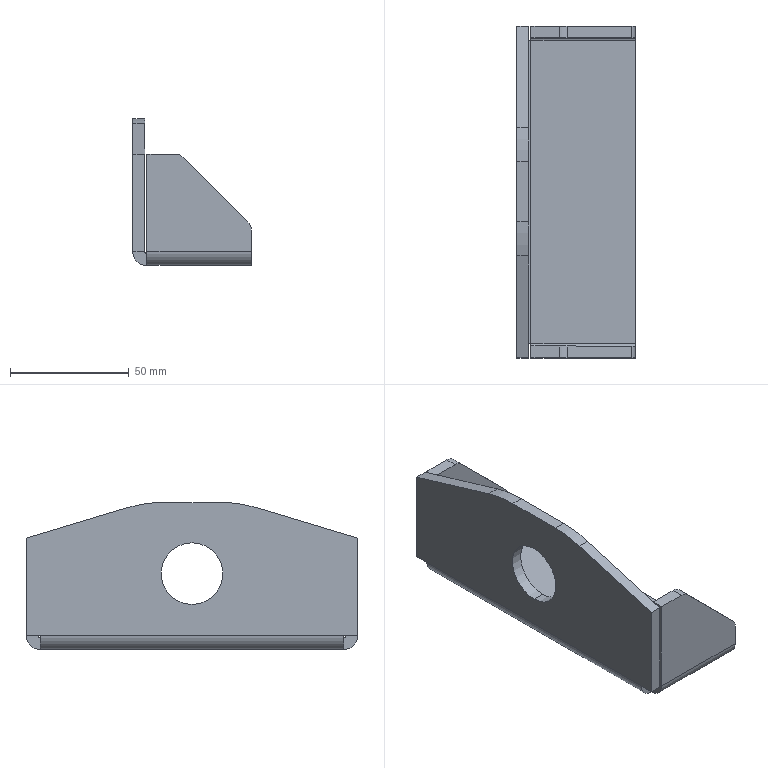Part | SolidWorks | features BaseBody 1 | 1 solid | 44 faces | box 50 x 140 x 62 mm | volume 80396 mm3 | plane 30 | cylinder 14 | commonest cylinder face diameters 10 x4 2 x3 12 x3 26 x2 100 x2
STEP:
#1=CARTESIAN_POINT('',(-20.,0.,14.));
#2=VERTEX_POINT('',#1);
#3=CARTESIAN_POINT('',(-25.,0.,14.));
#4=VERTEX_POINT('',#3);
#5=CARTESIAN_POINT('',(-20.,0.,14.));
#6=DIRECTION('',(-1.,0.,0.));
#7=VECTOR('',#6,1000.);
#8=LINE('',#5,#7);
#9=EDGE_CURVE('',#2,#4,#8,.T.);
#10=ORIENTED_EDGE('',*,*,#9,.F.);
#11=CARTESIAN_POINT('',(-20.,0.,40.));
#12=VERTEX_POINT('',#11);
#13=CARTESIAN_POINT('',(-20.,0.,27.));
#14=DIRECTION('',(-1.,0.,0.));
#15=DIRECTION('',(0.,0.,1.));
#16=AXIS2_PLACEMENT_3D('',#13,#14,#15);
#17=CIRCLE('',#16,13.);
#18=EDGE_CURVE('',#12,#2,#17,.T.);
#19=ORIENTED_EDGE('',*,*,#18,.F.);
#20=CARTESIAN_POINT('',(-25.,0.,40.));
#21=VERTEX_POINT('',#20);
#22=CARTESIAN_POINT('',(-20.,0.,40.));
#23=DIRECTION('',(-1.,0.,0.));
#24=VECTOR('',#23,1000.);
#25=LINE('',#22,#24);
#26=EDGE_CURVE('',#12,#21,#25,.T.);
#27=ORIENTED_EDGE('',*,*,#26,.T.);
#28=CARTESIAN_POINT('',(-25.,0.,27.));
#29=DIRECTION('',(-1.,0.,0.));
#30=DIRECTION('',(0.,0.,1.));
#31=AXIS2_PLACEMENT_3D('',#28,#29,#30);
#32=CIRCLE('',#31,13.);
#33=EDGE_CURVE('',#21,#4,#32,.T.);
#34=ORIENTED_EDGE('',*,*,#33,.T.);
#35=EDGE_LOOP('',(#10,#19,#27,#34));
#36=FACE_OUTER_BOUND('',#35,.T.);
#37=CARTESIAN_POINT('',(-20.,0.,27.));
#38=DIRECTION('',(-1.,0.,0.));
#39=DIRECTION('',(0.,0.,1.));
#40=AXIS2_PLACEMENT_3D('',#37,#38,#39);
#41=CYLINDRICAL_SURFACE('',#40,13.);
#42=ADVANCED_FACE('',(#36),#41,.F.);
#43=CARTESIAN_POINT('',(-3.536,-70.,40.536));
#44=VERTEX_POINT('',#43);
#45=CARTESIAN_POINT('',(-7.071,-70.,42.));
#46=VERTEX_POINT('',#45);
#47=CARTESIAN_POINT('',(-7.071,-70.,37.));
#48=DIRECTION('',(0.,-1.,0.));
#49=DIRECTION('',(0.,0.,1.));
#50=AXIS2_PLACEMENT_3D('',#47,#48,#49);
#51=CIRCLE('',#50,5.);
#52=EDGE_CURVE('',#44,#46,#51,.T.);
#53=ORIENTED_EDGE('',*,*,#52,.F.);
#54=CARTESIAN_POINT('',(-3.536,-65.,40.536));
#55=VERTEX_POINT('',#54);
#56=CARTESIAN_POINT('',(-3.536,-70.,40.536));
#57=DIRECTION('',(0.,-1.,0.));
#58=VECTOR('',#57,1000.);
#59=LINE('',#56,#58);
#60=EDGE_CURVE('',#55,#44,#59,.T.);
#61=ORIENTED_EDGE('',*,*,#60,.F.);
#62=CARTESIAN_POINT('',(-7.071,-65.,42.));
#63=VERTEX_POINT('',#62);
#64=CARTESIAN_POINT('',(-7.071,-65.,37.));
#65=DIRECTION('',(0.,1.,0.));
#66=DIRECTION('',(0.,0.,1.));
#67=AXIS2_PLACEMENT_3D('',#64,#65,#66);
#68=CIRCLE('',#67,5.);
#69=EDGE_CURVE('',#63,#55,#68,.T.);
#70=ORIENTED_EDGE('',*,*,#69,.F.);
#71=CARTESIAN_POINT('',(-7.071,-65.,42.));
#72=DIRECTION('',(0.,1.,0.));
#73=VECTOR('',#72,1000.);
#74=LINE('',#71,#73);
#75=EDGE_CURVE('',#46,#63,#74,.T.);
#76=ORIENTED_EDGE('',*,*,#75,.F.);
#77=EDGE_LOOP('',(#53,#61,#70,#76));
#78=FACE_OUTER_BOUND('',#77,.T.);
#79=CARTESIAN_POINT('',(-7.071,-70.,37.));
#80=DIRECTION('',(0.,1.,0.));
#81=DIRECTION('',(0.,0.,1.));
#82=AXIS2_PLACEMENT_3D('',#79,#80,#81);
#83=CYLINDRICAL_SURFACE('',#82,5.);
#84=ADVANCED_FACE('',(#78),#83,.T.);
#85=CARTESIAN_POINT('',(23.536,-65.,13.464));
#86=VERTEX_POINT('',#85);
#87=CARTESIAN_POINT('',(25.,-65.,9.929));
#88=VERTEX_POINT('',#87);
#89=CARTESIAN_POINT('',(20.,-65.,9.929));
#90=DIRECTION('',(0.,1.,0.));
#91=DIRECTION('',(0.,0.,1.));
#92=AXIS2_PLACEMENT_3D('',#89,#90,#91);
#93=CIRCLE('',#92,5.);
#94=EDGE_CURVE('',#86,#88,#93,.T.);
#95=ORIENTED_EDGE('',*,*,#94,.F.);
#96=CARTESIAN_POINT('',(23.536,-70.,13.464));
#97=VERTEX_POINT('',#96);
#98=CARTESIAN_POINT('',(23.536,-65.,13.464));
#99=DIRECTION('',(0.,1.,0.));
#100=VECTOR('',#99,1000.);
#101=LINE('',#98,#100);
#102=EDGE_CURVE('',#97,#86,#101,.T.);
#103=ORIENTED_EDGE('',*,*,#102,.F.);
#104=CARTESIAN_POINT('',(25.,-70.,9.929));
#105=VERTEX_POINT('',#104);
#106=CARTESIAN_POINT('',(20.,-70.,9.929));
#107=DIRECTION('',(0.,-1.,0.));
#108=DIRECTION('',(0.,0.,1.));
#109=AXIS2_PLACEMENT_3D('',#106,#107,#108);
#110=CIRCLE('',#109,5.);
#111=EDGE_CURVE('',#105,#97,#110,.T.);
#112=ORIENTED_EDGE('',*,*,#111,.F.);
#113=CARTESIAN_POINT('',(25.,-70.,9.929));
#114=DIRECTION('',(0.,-1.,0.));
#115=VECTOR('',#114,1000.);
#116=LINE('',#113,#115);
#117=EDGE_CURVE('',#88,#105,#116,.T.);
#118=ORIENTED_EDGE('',*,*,#117,.F.);
#119=EDGE_LOOP('',(#95,#103,#112,#118));
#120=FACE_OUTER_BOUND('',#119,.T.);
#121=CARTESIAN_POINT('',(20.,-70.,9.929));
#122=DIRECTION('',(0.,-1.,0.));
#123=DIRECTION('',(0.,0.,-1.));
#124=AXIS2_PLACEMENT_3D('',#121,#122,#123);
#125=CYLINDRICAL_SURFACE('',#124,5.);
#126=ADVANCED_FACE('',(#120),#125,.T.);
#127=CARTESIAN_POINT('',(23.536,70.,13.464));
#128=VERTEX_POINT('',#127);
#129=CARTESIAN_POINT('',(25.,70.,9.929));
#130=VERTEX_POINT('',#129);
#131=CARTESIAN_POINT('',(20.,70.,9.929));
#132=DIRECTION('',(0.,1.,0.));
#133=DIRECTION('',(0.,0.,-1.));
#134=AXIS2_PLACEMENT_3D('',#131,#132,#133);
#135=CIRCLE('',#134,5.);
#136=EDGE_CURVE('',#128,#130,#135,.T.);
#137=ORIENTED_EDGE('',*,*,#136,.F.);
#138=CARTESIAN_POINT('',(23.536,65.,13.464));
#139=VERTEX_POINT('',#138);
#140=CARTESIAN_POINT('',(23.536,70.,13.464));
#141=DIRECTION('',(0.,1.,0.));
#142=VECTOR('',#141,1000.);
#143=LINE('',#140,#142);
#144=EDGE_CURVE('',#139,#128,#143,.T.);
#145=ORIENTED_EDGE('',*,*,#144,.F.);
#146=CARTESIAN_POINT('',(25.,65.,9.929));
#147=VERTEX_POINT('',#146);
#148=CARTESIAN_POINT('',(20.,65.,9.929));
#149=DIRECTION('',(0.,-1.,0.));
#150=DIRECTION('',(0.,0.,-1.));
#151=AXIS2_PLACEMENT_3D('',#148,#149,#150);
#152=CIRCLE('',#151,5.);
#153=EDGE_CURVE('',#147,#139,#152,.T.);
#154=ORIENTED_EDGE('',*,*,#153,.F.);
#155=CARTESIAN_POINT('',(25.,65.,9.929));
#156=DIRECTION('',(0.,-1.,0.));
#157=VECTOR('',#156,1000.);
#158=LINE('',#155,#157);
#159=EDGE_CURVE('',#130,#147,#158,.T.);
#160=ORIENTED_EDGE('',*,*,#159,.F.);
#161=EDGE_LOOP('',(#137,#145,#154,#160));
#162=FACE_OUTER_BOUND('',#161,.T.);
#163=CARTESIAN_POINT('',(20.,70.,9.929));
#164=DIRECTION('',(0.,-1.,0.));
#165=DIRECTION('',(0.,0.,-1.));
#166=AXIS2_PLACEMENT_3D('',#163,#164,#165);
#167=CYLINDRICAL_SURFACE('',#166,5.);
#168=ADVANCED_FACE('',(#162),#167,.T.);
#169=CARTESIAN_POINT('',(-3.536,65.,40.536));
#170=VERTEX_POINT('',#169);
#171=CARTESIAN_POINT('',(-7.071,65.,42.));
#172=VERTEX_POINT('',#171);
#173=CARTESIAN_POINT('',(-7.071,65.,37.));
#174=DIRECTION('',(0.,-1.,0.));
#175=DIRECTION('',(0.,0.,-1.));
#176=AXIS2_PLACEMENT_3D('',#173,#174,#175);
#177=CIRCLE('',#176,5.);
#178=EDGE_CURVE('',#170,#172,#177,.T.);
#179=ORIENTED_EDGE('',*,*,#178,.F.);
#180=CARTESIAN_POINT('',(-3.536,70.,40.536));
#181=VERTEX_POINT('',#180);
#182=CARTESIAN_POINT('',(-3.536,65.,40.536));
#183=DIRECTION('',(0.,-1.,0.));
#184=VECTOR('',#183,1000.);
#185=LINE('',#182,#184);
#186=EDGE_CURVE('',#181,#170,#185,.T.);
#187=ORIENTED_EDGE('',*,*,#186,.F.);
#188=CARTESIAN_POINT('',(-7.071,70.,42.));
#189=VERTEX_POINT('',#188);
#190=CARTESIAN_POINT('',(-7.071,70.,37.));
#191=DIRECTION('',(0.,1.,0.));
#192=DIRECTION('',(0.,0.,-1.));
#193=AXIS2_PLACEMENT_3D('',#190,#191,#192);
#194=CIRCLE('',#193,5.);
#195=EDGE_CURVE('',#189,#181,#194,.T.);
#196=ORIENTED_EDGE('',*,*,#195,.F.);
#197=CARTESIAN_POINT('',(-7.071,70.,42.));
#198=DIRECTION('',(0.,1.,0.));
#199=VECTOR('',#198,1000.);
#200=LINE('',#197,#199);
#201=EDGE_CURVE('',#172,#189,#200,.T.);
#202=ORIENTED_EDGE('',*,*,#201,.F.);
#203=EDGE_LOOP('',(#179,#187,#196,#202));
#204=FACE_OUTER_BOUND('',#203,.T.);
#205=CARTESIAN_POINT('',(-7.071,70.,37.));
#206=DIRECTION('',(0.,1.,0.));
#207=DIRECTION('',(0.,0.,1.));
#208=AXIS2_PLACEMENT_3D('',#205,#206,#207);
#209=CYLINDRICAL_SURFACE('',#208,5.);
#210=ADVANCED_FACE('',(#204),#209,.T.);
#211=CARTESIAN_POINT('',(-25.,-27.029,54.891));
#212=VERTEX_POINT('',#211);
#213=CARTESIAN_POINT('',(-25.,-12.662,57.));
#214=VERTEX_POINT('',#213);
#215=CARTESIAN_POINT('',(-25.,-12.662,7.));
#216=DIRECTION('',(-1.,0.,0.));
#217=DIRECTION('',(0.,0.,-1.));
#218=AXIS2_PLACEMENT_3D('',#215,#216,#217);
#219=CIRCLE('',#218,50.);
#220=EDGE_CURVE('',#212,#214,#219,.T.);
#221=ORIENTED_EDGE('',*,*,#220,.F.);
#222=CARTESIAN_POINT('',(-20.,-27.029,54.891));
#223=VERTEX_POINT('',#222);
#224=CARTESIAN_POINT('',(-25.,-27.029,54.891));
#225=DIRECTION('',(-1.,0.,0.));
#226=VECTOR('',#225,1000.);
#227=LINE('',#224,#226);
#228=EDGE_CURVE('',#223,#212,#227,.T.);
#229=ORIENTED_EDGE('',*,*,#228,.F.);
#230=CARTESIAN_POINT('',(-20.,-12.662,57.));
#231=VERTEX_POINT('',#230);
#232=CARTESIAN_POINT('',(-20.,-12.662,7.));
#233=DIRECTION('',(1.,0.,0.));
#234=DIRECTION('',(0.,0.,-1.));
#235=AXIS2_PLACEMENT_3D('',#232,#233,#234);
#236=CIRCLE('',#235,50.);
#237=EDGE_CURVE('',#231,#223,#236,.T.);
#238=ORIENTED_EDGE('',*,*,#237,.F.);
#239=CARTESIAN_POINT('',(-20.,-12.662,57.));
#240=DIRECTION('',(1.,0.,0.));
#241=VECTOR('',#240,1000.);
#242=LINE('',#239,#241);
#243=EDGE_CURVE('',#214,#231,#242,.T.);
#244=ORIENTED_EDGE('',*,*,#243,.F.);
#245=EDGE_LOOP('',(#221,#229,#238,#244));
#246=FACE_OUTER_BOUND('',#245,.T.);
#247=CARTESIAN_POINT('',(-25.,-12.662,7.));
#248=DIRECTION('',(1.,0.,0.));
#249=DIRECTION('',(0.,0.,-1.));
#250=AXIS2_PLACEMENT_3D('',#247,#248,#249);
#251=CYLINDRICAL_SURFACE('',#250,50.);
#252=ADVANCED_FACE('',(#246),#251,.T.);
#253=CARTESIAN_POINT('',(-20.,27.029,54.891));
#254=VERTEX_POINT('',#253);
#255=CARTESIAN_POINT('',(-20.,12.662,57.));
#256=VERTEX_POINT('',#255);
#257=CARTESIAN_POINT('',(-20.,12.662,7.));
#258=DIRECTION('',(1.,0.,0.));
#259=DIRECTION('',(0.,0.,-1.));
#260=AXIS2_PLACEMENT_3D('',#257,#258,#259);
#261=CIRCLE('',#260,50.);
#262=EDGE_CURVE('',#254,#256,#261,.T.);
#263=ORIENTED_EDGE('',*,*,#262,.F.);
#264=CARTESIAN_POINT('',(-25.,27.029,54.891));
#265=VERTEX_POINT('',#264);
#266=CARTESIAN_POINT('',(-20.,27.029,54.891));
#267=DIRECTION('',(1.,0.,0.));
#268=VECTOR('',#267,1000.);
#269=LINE('',#266,#268);
#270=EDGE_CURVE('',#265,#254,#269,.T.);
#271=ORIENTED_EDGE('',*,*,#270,.F.);
#272=CARTESIAN_POINT('',(-25.,12.662,57.));
#273=VERTEX_POINT('',#272);
#274=CARTESIAN_POINT('',(-25.,12.662,7.));
#275=DIRECTION('',(-1.,0.,0.));
#276=DIRECTION('',(0.,0.,-1.));
#277=AXIS2_PLACEMENT_3D('',#274,#275,#276);
#278=CIRCLE('',#277,50.);
#279=EDGE_CURVE('',#273,#265,#278,.T.);
#280=ORIENTED_EDGE('',*,*,#279,.F.);
#281=CARTESIAN_POINT('',(-25.,12.662,57.));
#282=DIRECTION('',(-1.,0.,0.));
#283=VECTOR('',#282,1000.);
#284=LINE('',#281,#283);
#285=EDGE_CURVE('',#256,#273,#284,.T.);
#286=ORIENTED_EDGE('',*,*,#285,.F.);
#287=EDGE_LOOP('',(#263,#271,#280,#286));
#288=FACE_OUTER_BOUND('',#287,.T.);
#289=CARTESIAN_POINT('',(-25.,12.662,7.));
#290=DIRECTION('',(-1.,0.,0.));
#291=DIRECTION('',(0.,0.,1.));
#292=AXIS2_PLACEMENT_3D('',#289,#290,#291);
#293=CYLINDRICAL_SURFACE('',#292,50.);
#294=ADVANCED_FACE('',(#288),#293,.T.);
#295=CARTESIAN_POINT('',(-20.,-70.,42.));
#296=VERTEX_POINT('',#295);
#297=CARTESIAN_POINT('',(-20.,-17.339,57.798));
#298=DIRECTION('',(0.,-0.9578,-0.2873));
#299=VECTOR('',#298,1000.);
#300=LINE('',#297,#299);
#301=EDGE_CURVE('',#223,#296,#300,.T.);
#302=ORIENTED_EDGE('',*,*,#301,.F.);
#303=ORIENTED_EDGE('',*,*,#228,.T.);
#304=CARTESIAN_POINT('',(-25.,-70.,42.));
#305=VERTEX_POINT('',#304);
#306=CARTESIAN_POINT('',(-25.,-20.,57.));
#307=DIRECTION('',(0.,0.9578,0.2873));
#308=VECTOR('',#307,1000.);
#309=LINE('',#306,#308);
#310=EDGE_CURVE('',#305,#212,#309,.T.);
#311=ORIENTED_EDGE('',*,*,#310,.F.);
#312=CARTESIAN_POINT('',(-25.,-70.,42.));
#313=DIRECTION('',(-1.,0.,0.));
#314=VECTOR('',#313,1000.);
#315=LINE('',#312,#314);
#316=EDGE_CURVE('',#296,#305,#315,.T.);
#317=ORIENTED_EDGE('',*,*,#316,.F.);
#318=EDGE_LOOP('',(#302,#303,#311,#317));
#319=FACE_OUTER_BOUND('',#318,.T.);
#320=CARTESIAN_POINT('',(-25.,-20.,57.));
#321=DIRECTION('',(0.,0.2873,-0.9578));
#322=DIRECTION('',(-1.,0.,0.));
#323=AXIS2_PLACEMENT_3D('',#320,#321,#322);
#324=PLANE('',#323);
#325=ADVANCED_FACE('',(#319),#324,.F.);
#326=CARTESIAN_POINT('',(-25.,70.,42.));
#327=VERTEX_POINT('',#326);
#328=CARTESIAN_POINT('',(-25.,70.,42.));
#329=DIRECTION('',(0.,0.9578,-0.2873));
#330=VECTOR('',#329,1000.);
#331=LINE('',#328,#330);
#332=EDGE_CURVE('',#265,#327,#331,.T.);
#333=ORIENTED_EDGE('',*,*,#332,.F.);
#334=ORIENTED_EDGE('',*,*,#270,.T.);
#335=CARTESIAN_POINT('',(-20.,70.,42.));
#336=VERTEX_POINT('',#335);
#337=CARTESIAN_POINT('',(-20.,17.339,57.798));
#338=DIRECTION('',(0.,-0.9578,0.2873));
#339=VECTOR('',#338,1000.);
#340=LINE('',#337,#339);
#341=EDGE_CURVE('',#336,#254,#340,.T.);
#342=ORIENTED_EDGE('',*,*,#341,.F.);
#343=CARTESIAN_POINT('',(-25.,70.,42.));
#344=DIRECTION('',(1.,0.,0.));
#345=VECTOR('',#344,1000.);
#346=LINE('',#343,#345);
#347=EDGE_CURVE('',#327,#336,#346,.T.);
#348=ORIENTED_EDGE('',*,*,#347,.F.);
#349=EDGE_LOOP('',(#333,#334,#342,#348));
#350=FACE_OUTER_BOUND('',#349,.T.);
#351=CARTESIAN_POINT('',(-25.,70.,42.));
#352=DIRECTION('',(0.,-0.2873,-0.9578));
#353=DIRECTION('',(0.,-0.9578,0.2873));
#354=AXIS2_PLACEMENT_3D('',#351,#352,#353);
#355=PLANE('',#354);
#356=ADVANCED_FACE('',(#350),#355,.F.);
#357=CARTESIAN_POINT('',(-5.,-70.,42.));
#358=DIRECTION('',(-0.7071,0.,0.7071));
#359=VECTOR('',#358,1000.);
#360=LINE('',#357,#359);
#361=EDGE_CURVE('',#97,#44,#360,.T.);
#362=ORIENTED_EDGE('',*,*,#361,.F.);
#363=ORIENTED_EDGE('',*,*,#102,.T.);
#364=CARTESIAN_POINT('',(18.5,-65.,18.5));
#365=DIRECTION('',(0.7071,0.,-0.7071));
#366=VECTOR('',#365,1000.);
#367=LINE('',#364,#366);
#368=EDGE_CURVE('',#55,#86,#367,.T.);
#369=ORIENTED_EDGE('',*,*,#368,.F.);
#370=ORIENTED_EDGE('',*,*,#60,.T.);
#371=EDGE_LOOP('',(#362,#363,#369,#370));
#372=FACE_OUTER_BOUND('',#371,.T.);
#373=CARTESIAN_POINT('',(-5.,-70.,42.));
#374=DIRECTION('',(-0.7071,0.,-0.7071));
#375=DIRECTION('',(-0.7071,0.,0.7071));
#376=AXIS2_PLACEMENT_3D('',#373,#374,#375);
#377=PLANE('',#376);
#378=ADVANCED_FACE('',(#372),#377,.F.);
#379=CARTESIAN_POINT('',(25.,70.,12.));
#380=DIRECTION('',(0.7071,0.,-0.7071));
#381=VECTOR('',#380,1000.);
#382=LINE('',#379,#381);
#383=EDGE_CURVE('',#181,#128,#382,.T.);
#384=ORIENTED_EDGE('',*,*,#383,.F.);
#385=ORIENTED_EDGE('',*,*,#186,.T.);
#386=CARTESIAN_POINT('',(18.5,65.,18.5));
#387=DIRECTION('',(-0.7071,0.,0.7071));
#388=VECTOR('',#387,1000.);
#389=LINE('',#386,#388);
#390=EDGE_CURVE('',#139,#170,#389,.T.);
#391=ORIENTED_EDGE('',*,*,#390,.F.);
#392=ORIENTED_EDGE('',*,*,#144,.T.);
#393=EDGE_LOOP('',(#384,#385,#391,#392));
#394=FACE_OUTER_BOUND('',#393,.T.);
#395=CARTESIAN_POINT('',(25.,70.,12.));
#396=DIRECTION('',(-0.7071,0.,-0.7071));
#397=DIRECTION('',(-0.7071,0.,0.7071));
#398=AXIS2_PLACEMENT_3D('',#395,#396,#397);
#399=PLANE('',#398);
#400=ADVANCED_FACE('',(#394),#399,.F.);
#401=CARTESIAN_POINT('',(-19.,65.,42.));
#402=VERTEX_POINT('',#401);
#403=CARTESIAN_POINT('',(25.,65.,42.));
#404=DIRECTION('',(1.,0.,0.));
#405=VECTOR('',#404,1000.);
#406=LINE('',#403,#405);
#407=EDGE_CURVE('',#402,#172,#406,.T.);
#408=ORIENTED_EDGE('',*,*,#407,.T.);
#409=ORIENTED_EDGE('',*,*,#201,.T.);
#410=CARTESIAN_POINT('',(-19.,70.,42.));
#411=VERTEX_POINT('',#410);
#412=CARTESIAN_POINT('',(0.,70.,42.));
#413=DIRECTION('',(1.,0.,0.));
#414=VECTOR('',#413,1000.);
#415=LINE('',#412,#414);
#416=EDGE_CURVE('',#411,#189,#415,.T.);
#417=ORIENTED_EDGE('',*,*,#416,.F.);
#418=CARTESIAN_POINT('',(-19.,70.,42.));
#419=DIRECTION('',(0.,-1.,0.));
#420=VECTOR('',#419,1000.);
#421=LINE('',#418,#420);
#422=EDGE_CURVE('',#411,#402,#421,.T.);
#423=ORIENTED_EDGE('',*,*,#422,.T.);
#424=EDGE_LOOP('',(#408,#409,#417,#423));
#425=FACE_OUTER_BOUND('',#424,.T.);
#426=CARTESIAN_POINT('',(25.,70.,42.));
#427=DIRECTION('',(0.,0.,-1.));
#428=DIRECTION('',(0.,-1.,0.));
#429=AXIS2_PLACEMENT_3D('',#426,#427,#428);
#430=PLANE('',#429);
#431=ADVANCED_FACE('',(#425),#430,.F.);
#432=ORIENTED_EDGE('',*,*,#390,.T.);
#433=ORIENTED_EDGE('',*,*,#178,.T.);
#434=ORIENTED_EDGE('',*,*,#407,.F.);
#435=CARTESIAN_POINT('',(-19.,65.,1.));
#436=VERTEX_POINT('',#435);
#437=CARTESIAN_POINT('',(-19.,65.,42.));
#438=DIRECTION('',(0.,0.,1.));
#439=VECTOR('',#438,1000.);
#440=LINE('',#437,#439);
#441=EDGE_CURVE('',#436,#402,#440,.T.);
#442=ORIENTED_EDGE('',*,*,#441,.F.);
#443=CARTESIAN_POINT('',(25.,65.,1.));
#444=VERTEX_POINT('',#443);
#445=CARTESIAN_POINT('',(25.,65.,1.));
#446=DIRECTION('',(-1.,0.,0.));
#447=VECTOR('',#446,1000.);
#448=LINE('',#445,#447);
#449=EDGE_CURVE('',#444,#436,#448,.T.);
#450=ORIENTED_EDGE('',*,*,#449,.F.);
#451=CARTESIAN_POINT('',(25.,65.,0.));
#452=DIRECTION('',(0.,0.,-1.));
#453=VECTOR('',#452,1000.);
#454=LINE('',#451,#453);
#455=EDGE_CURVE('',#147,#444,#454,.T.);
#456=ORIENTED_EDGE('',*,*,#455,.F.);
#457=ORIENTED_EDGE('',*,*,#153,.T.);
#458=EDGE_LOOP('',(#432,#433,#434,#442,#450,#456,#457));
#459=FACE_OUTER_BOUND('',#458,.T.);
#460=CARTESIAN_POINT('',(0.,65.,0.));
#461=DIRECTION('',(0.,-1.,0.));
#462=DIRECTION('',(-1.,0.,0.));
#463=AXIS2_PLACEMENT_3D('',#460,#461,#462);
#464=PLANE('',#463);
#465=ADVANCED_FACE('',(#459),#464,.T.);
#466=ORIENTED_EDGE('',*,*,#416,.T.);
#467=ORIENTED_EDGE('',*,*,#195,.T.);
#468=ORIENTED_EDGE('',*,*,#383,.T.);
#469=ORIENTED_EDGE('',*,*,#136,.T.);
#470=CARTESIAN_POINT('',(25.,70.,1.));
#471=VERTEX_POINT('',#470);
#472=CARTESIAN_POINT('',(25.,70.,0.));
#473=DIRECTION('',(0.,0.,-1.));
#474=VECTOR('',#473,1000.);
#475=LINE('',#472,#474);
#476=EDGE_CURVE('',#130,#471,#475,.T.);
#477=ORIENTED_EDGE('',*,*,#476,.T.);
#478=CARTESIAN_POINT('',(-19.,70.,1.));
#479=VERTEX_POINT('',#478);
#480=CARTESIAN_POINT('',(25.,70.,1.));
#481=DIRECTION('',(1.,0.,0.));
#482=VECTOR('',#481,1000.);
#483=LINE('',#480,#482);
#484=EDGE_CURVE('',#479,#471,#483,.T.);
#485=ORIENTED_EDGE('',*,*,#484,.F.);
#486=CARTESIAN_POINT('',(-19.,70.,0.));
#487=DIRECTION('',(0.,0.,1.));
#488=VECTOR('',#487,1000.);
#489=LINE('',#486,#488);
#490=EDGE_CURVE('',#479,#411,#489,.T.);
#491=ORIENTED_EDGE('',*,*,#490,.T.);
#492=EDGE_LOOP('',(#466,#467,#468,#469,#477,#485,#491));
#493=FACE_OUTER_BOUND('',#492,.T.);
#494=CARTESIAN_POINT('',(0.,70.,0.));
#495=DIRECTION('',(0.,-1.,0.));
#496=DIRECTION('',(-1.,0.,0.));
#497=AXIS2_PLACEMENT_3D('',#494,#495,#496);
#498=PLANE('',#497);
#499=ADVANCED_FACE('',(#493),#498,.F.);
#500=CARTESIAN_POINT('',(-19.,65.,1.));
#501=DIRECTION('',(0.,1.,0.));
#502=VECTOR('',#501,1000.);
#503=LINE('',#500,#502);
#504=EDGE_CURVE('',#436,#479,#503,.T.);
#505=ORIENTED_EDGE('',*,*,#504,.F.);
#506=ORIENTED_EDGE('',*,*,#441,.T.);
#507=ORIENTED_EDGE('',*,*,#422,.F.);
#508=ORIENTED_EDGE('',*,*,#490,.F.);
#509=EDGE_LOOP('',(#505,#506,#507,#508));
#510=FACE_OUTER_BOUND('',#509,.T.);
#511=CARTESIAN_POINT('',(-19.,70.,42.));
#512=DIRECTION('',(1.,0.,0.));
#513=DIRECTION('',(0.,1.,0.));
#514=AXIS2_PLACEMENT_3D('',#511,#512,#513);
#515=PLANE('',#514);
#516=ADVANCED_FACE('',(#510),#515,.F.);
#517=ORIENTED_EDGE('',*,*,#476,.F.);
#518=ORIENTED_EDGE('',*,*,#159,.T.);
#519=ORIENTED_EDGE('',*,*,#455,.T.);
#520=CARTESIAN_POINT('',(25.,70.,1.));
#521=DIRECTION('',(0.,1.,0.));
#522=VECTOR('',#521,1000.);
#523=LINE('',#520,#522);
#524=EDGE_CURVE('',#444,#471,#523,.T.);
#525=ORIENTED_EDGE('',*,*,#524,.T.);
#526=EDGE_LOOP('',(#517,#518,#519,#525));
#527=FACE_OUTER_BOUND('',#526,.T.);
#528=CARTESIAN_POINT('',(25.,70.,0.));
#529=DIRECTION('',(-1.,0.,0.));
#530=DIRECTION('',(0.,1.,0.));
#531=AXIS2_PLACEMENT_3D('',#528,#529,#530);
#532=PLANE('',#531);
#533=ADVANCED_FACE('',(#527),#532,.F.);
#534=CARTESIAN_POINT('',(-19.,64.,0.));
#535=VERTEX_POINT('',#534);
#536=CARTESIAN_POINT('',(25.,64.,0.));
#537=VERTEX_POINT('',#536);
#538=CARTESIAN_POINT('',(-19.,64.,0.));
#539=DIRECTION('',(1.,0.,0.));
#540=VECTOR('',#539,1000.);
#541=LINE('',#538,#540);
#542=EDGE_CURVE('',#535,#537,#541,.T.);
#543=ORIENTED_EDGE('',*,*,#542,.T.);
#544=CARTESIAN_POINT('',(25.,64.,1.));
#545=DIRECTION('',(1.,0.,0.));
#546=DIRECTION('',(0.,0.,1.));
#547=AXIS2_PLACEMENT_3D('',#544,#545,#546);
#548=CIRCLE('',#547,1.);
#549=EDGE_CURVE('',#537,#444,#548,.T.);
#550=ORIENTED_EDGE('',*,*,#549,.T.);
#551=ORIENTED_EDGE('',*,*,#449,.T.);
#552=CARTESIAN_POINT('',(-19.,64.,1.));
#553=DIRECTION('',(-1.,0.,0.));
#554=DIRECTION('',(0.,0.,1.));
#555=AXIS2_PLACEMENT_3D('',#552,#553,#554);
#556=CIRCLE('',#555,1.);
#557=EDGE_CURVE('',#436,#535,#556,.T.);
#558=ORIENTED_EDGE('',*,*,#557,.T.);
#559=EDGE_LOOP('',(#543,#550,#551,#558));
#560=FACE_OUTER_BOUND('',#559,.T.);
#561=CARTESIAN_POINT('',(-19.,64.,1.));
#562=DIRECTION('',(-1.,0.,0.));
#563=DIRECTION('',(0.,1.,0.));
#564=AXIS2_PLACEMENT_3D('',#561,#562,#563);
#565=CYLINDRICAL_SURFACE('',#564,1.);
#566=ADVANCED_FACE('',(#560),#565,.F.);
#567=CARTESIAN_POINT('',(-19.,64.,-5.));
#568=VERTEX_POINT('',#567);
#569=CARTESIAN_POINT('',(25.,64.,-5.));
#570=VERTEX_POINT('',#569);
#571=CARTESIAN_POINT('',(-19.,64.,-5.));
#572=DIRECTION('',(1.,0.,0.));
#573=VECTOR('',#572,1000.);
#574=LINE('',#571,#573);
#575=EDGE_CURVE('',#568,#570,#574,.T.);
#576=ORIENTED_EDGE('',*,*,#575,.F.);
#577=CARTESIAN_POINT('',(-19.,64.,1.));
#578=DIRECTION('',(-1.,0.,0.));
#579=DIRECTION('',(0.,0.,1.));
#580=AXIS2_PLACEMENT_3D('',#577,#578,#579);
#581=CIRCLE('',#580,6.);
#582=EDGE_CURVE('',#479,#568,#581,.T.);
#583=ORIENTED_EDGE('',*,*,#582,.F.);
#584=ORIENTED_EDGE('',*,*,#484,.T.);
#585=CARTESIAN_POINT('',(25.,64.,1.));
#586=DIRECTION('',(1.,0.,0.));
#587=DIRECTION('',(0.,0.,1.));
#588=AXIS2_PLACEMENT_3D('',#585,#586,#587);
#589=CIRCLE('',#588,6.);
#590=EDGE_CURVE('',#570,#471,#589,.T.);
#591=ORIENTED_EDGE('',*,*,#590,.F.);
#592=EDGE_LOOP('',(#576,#583,#584,#591));
#593=FACE_OUTER_BOUND('',#592,.T.);
#594=CARTESIAN_POINT('',(-19.,64.,1.));
#595=DIRECTION('',(-1.,0.,0.));
#596=DIRECTION('',(0.,1.,0.));
#597=AXIS2_PLACEMENT_3D('',#594,#595,#596);
#598=CYLINDRICAL_SURFACE('',#597,6.);
#599=ADVANCED_FACE('',(#593),#598,.T.);
#600=ORIENTED_EDGE('',*,*,#557,.F.);
#601=ORIENTED_EDGE('',*,*,#504,.T.);
#602=ORIENTED_EDGE('',*,*,#582,.T.);
#603=CARTESIAN_POINT('',(-19.,64.,0.));
#604=DIRECTION('',(0.,0.,-1.));
#605=VECTOR('',#604,1000.);
#606=LINE('',#603,#605);
#607=EDGE_CURVE('',#535,#568,#606,.T.);
#608=ORIENTED_EDGE('',*,*,#607,.F.);
#609=EDGE_LOOP('',(#600,#601,#602,#608));
#610=FACE_OUTER_BOUND('',#609,.T.);
#611=CARTESIAN_POINT('',(-19.,64.,1.));
#612=DIRECTION('',(1.,0.,0.));
#613=DIRECTION('',(0.,0.,1.));
#614=AXIS2_PLACEMENT_3D('',#611,#612,#613);
#615=PLANE('',#614);
#616=ADVANCED_FACE('',(#610),#615,.F.);
#617=ORIENTED_EDGE('',*,*,#524,.F.);
#618=ORIENTED_EDGE('',*,*,#549,.F.);
#619=CARTESIAN_POINT('',(25.,64.,0.));
#620=DIRECTION('',(0.,0.,-1.));
#621=VECTOR('',#620,1000.);
#622=LINE('',#619,#621);
#623=EDGE_CURVE('',#537,#570,#622,.T.);
#624=ORIENTED_EDGE('',*,*,#623,.T.);
#625=ORIENTED_EDGE('',*,*,#590,.T.);
#626=EDGE_LOOP('',(#617,#618,#624,#625));
#627=FACE_OUTER_BOUND('',#626,.T.);
#628=CARTESIAN_POINT('',(25.,64.,1.));
#629=DIRECTION('',(1.,0.,0.));
#630=DIRECTION('',(0.,0.,1.));
#631=AXIS2_PLACEMENT_3D('',#628,#629,#630);
#632=PLANE('',#631);
#633=ADVANCED_FACE('',(#627),#632,.T.);
#634=CARTESIAN_POINT('',(-19.,-70.,42.));
#635=VERTEX_POINT('',#634);
#636=CARTESIAN_POINT('',(0.,-70.,42.));
#637=DIRECTION('',(-1.,0.,0.));
#638=VECTOR('',#637,1000.);
#639=LINE('',#636,#638);
#640=EDGE_CURVE('',#46,#635,#639,.T.);
#641=ORIENTED_EDGE('',*,*,#640,.F.);
#642=ORIENTED_EDGE('',*,*,#75,.T.);
#643=CARTESIAN_POINT('',(-19.,-65.,42.));
#644=VERTEX_POINT('',#643);
#645=CARTESIAN_POINT('',(-19.,-65.,42.));
#646=DIRECTION('',(-1.,0.,0.));
#647=VECTOR('',#646,1000.);
#648=LINE('',#645,#647);
#649=EDGE_CURVE('',#63,#644,#648,.T.);
#650=ORIENTED_EDGE('',*,*,#649,.T.);
#651=CARTESIAN_POINT('',(-19.,-70.,42.));
#652=DIRECTION('',(0.,1.,0.));
#653=VECTOR('',#652,1000.);
#654=LINE('',#651,#653);
#655=EDGE_CURVE('',#635,#644,#654,.T.);
#656=ORIENTED_EDGE('',*,*,#655,.F.);
#657=EDGE_LOOP('',(#641,#642,#650,#656));
#658=FACE_OUTER_BOUND('',#657,.T.);
#659=CARTESIAN_POINT('',(-19.,-70.,42.));
#660=DIRECTION('',(0.,0.,-1.));
#661=DIRECTION('',(-1.,0.,0.));
#662=AXIS2_PLACEMENT_3D('',#659,#660,#661);
#663=PLANE('',#662);
#664=ADVANCED_FACE('',(#658),#663,.F.);
#665=ORIENTED_EDGE('',*,*,#368,.T.);
#666=ORIENTED_EDGE('',*,*,#94,.T.);
#667=CARTESIAN_POINT('',(25.,-65.,1.));
#668=VERTEX_POINT('',#667);
#669=CARTESIAN_POINT('',(25.,-65.,42.));
#670=DIRECTION('',(0.,0.,1.));
#671=VECTOR('',#670,1000.);
#672=LINE('',#669,#671);
#673=EDGE_CURVE('',#668,#88,#672,.T.);
#674=ORIENTED_EDGE('',*,*,#673,.F.);
#675=CARTESIAN_POINT('',(-19.,-65.,1.));
#676=VERTEX_POINT('',#675);
#677=CARTESIAN_POINT('',(-19.,-65.,1.));
#678=DIRECTION('',(1.,0.,0.));
#679=VECTOR('',#678,1000.);
#680=LINE('',#677,#679);
#681=EDGE_CURVE('',#676,#668,#680,.T.);
#682=ORIENTED_EDGE('',*,*,#681,.F.);
#683=CARTESIAN_POINT('',(-19.,-65.,0.));
#684=DIRECTION('',(0.,0.,-1.));
#685=VECTOR('',#684,1000.);
#686=LINE('',#683,#685);
#687=EDGE_CURVE('',#644,#676,#686,.T.);
#688=ORIENTED_EDGE('',*,*,#687,.F.);
#689=ORIENTED_EDGE('',*,*,#649,.F.);
#690=ORIENTED_EDGE('',*,*,#69,.T.);
#691=EDGE_LOOP('',(#665,#666,#674,#682,#688,#689,#690));
#692=FACE_OUTER_BOUND('',#691,.T.);
#693=CARTESIAN_POINT('',(0.,-65.,0.));
#694=DIRECTION('',(0.,1.,0.));
#695=DIRECTION('',(0.,0.,-1.));
#696=AXIS2_PLACEMENT_3D('',#693,#694,#695);
#697=PLANE('',#696);
#698=ADVANCED_FACE('',(#692),#697,.T.);
#699=CARTESIAN_POINT('',(25.,-70.,1.));
#700=VERTEX_POINT('',#699);
#701=CARTESIAN_POINT('',(25.,-70.,0.));
#702=DIRECTION('',(0.,0.,1.));
#703=VECTOR('',#702,1000.);
#704=LINE('',#701,#703);
#705=EDGE_CURVE('',#700,#105,#704,.T.);
#706=ORIENTED_EDGE('',*,*,#705,.T.);
#707=ORIENTED_EDGE('',*,*,#111,.T.);
#708=ORIENTED_EDGE('',*,*,#361,.T.);
#709=ORIENTED_EDGE('',*,*,#52,.T.);
#710=ORIENTED_EDGE('',*,*,#640,.T.);
#711=CARTESIAN_POINT('',(-19.,-70.,1.));
#712=VERTEX_POINT('',#711);
#713=CARTESIAN_POINT('',(-19.,-70.,0.));
#714=DIRECTION('',(0.,0.,-1.));
#715=VECTOR('',#714,1000.);
#716=LINE('',#713,#715);
#717=EDGE_CURVE('',#635,#712,#716,.T.);
#718=ORIENTED_EDGE('',*,*,#717,.T.);
#719=CARTESIAN_POINT('',(-19.,-70.,1.));
#720=DIRECTION('',(-1.,0.,0.));
#721=VECTOR('',#720,1000.);
#722=LINE('',#719,#721);
#723=EDGE_CURVE('',#700,#712,#722,.T.);
#724=ORIENTED_EDGE('',*,*,#723,.F.);
#725=EDGE_LOOP('',(#706,#707,#708,#709,#710,#718,#724));
#726=FACE_OUTER_BOUND('',#725,.T.);
#727=CARTESIAN_POINT('',(0.,-70.,0.));
#728=DIRECTION('',(0.,1.,0.));
#729=DIRECTION('',(0.,0.,-1.));
#730=AXIS2_PLACEMENT_3D('',#727,#728,#729);
#731=PLANE('',#730);
#732=ADVANCED_FACE('',(#726),#731,.F.);
#733=ORIENTED_EDGE('',*,*,#673,.T.);
#734=ORIENTED_EDGE('',*,*,#117,.T.);
#735=ORIENTED_EDGE('',*,*,#705,.F.);
#736=CARTESIAN_POINT('',(25.,-65.,1.));
#737=DIRECTION('',(0.,-1.,0.));
#738=VECTOR('',#737,1000.);
#739=LINE('',#736,#738);
#740=EDGE_CURVE('',#668,#700,#739,.T.);
#741=ORIENTED_EDGE('',*,*,#740,.F.);
#742=EDGE_LOOP('',(#733,#734,#735,#741));
#743=FACE_OUTER_BOUND('',#742,.T.);
#744=CARTESIAN_POINT('',(25.,-70.,42.));
#745=DIRECTION('',(-1.,0.,0.));
#746=DIRECTION('',(0.,0.,1.));
#747=AXIS2_PLACEMENT_3D('',#744,#745,#746);
#748=PLANE('',#747);
#749=ADVANCED_FACE('',(#743),#748,.F.);
#750=CARTESIAN_POINT('',(-19.,-70.,1.));
#751=DIRECTION('',(0.,-1.,0.));
#752=VECTOR('',#751,1000.);
#753=LINE('',#750,#752);
#754=EDGE_CURVE('',#676,#712,#753,.T.);
#755=ORIENTED_EDGE('',*,*,#754,.T.);
#756=ORIENTED_EDGE('',*,*,#717,.F.);
#757=ORIENTED_EDGE('',*,*,#655,.T.);
#758=ORIENTED_EDGE('',*,*,#687,.T.);
#759=EDGE_LOOP('',(#755,#756,#757,#758));
#760=FACE_OUTER_BOUND('',#759,.T.);
#761=CARTESIAN_POINT('',(-19.,-70.,0.));
#762=DIRECTION('',(1.,0.,0.));
#763=DIRECTION('',(0.,0.,1.));
#764=AXIS2_PLACEMENT_3D('',#761,#762,#763);
#765=PLANE('',#764);
#766=ADVANCED_FACE('',(#760),#765,.F.);
#767=CARTESIAN_POINT('',(25.,-64.,0.));
#768=VERTEX_POINT('',#767);
#769=CARTESIAN_POINT('',(-19.,-64.,0.));
#770=VERTEX_POINT('',#769);
#771=CARTESIAN_POINT('',(25.,-64.,0.));
#772=DIRECTION('',(-1.,0.,0.));
#773=VECTOR('',#772,1000.);
#774=LINE('',#771,#773);
#775=EDGE_CURVE('',#768,#770,#774,.T.);
#776=ORIENTED_EDGE('',*,*,#775,.T.);
#777=CARTESIAN_POINT('',(-19.,-64.,1.));
#778=DIRECTION('',(-1.,0.,0.));
#779=DIRECTION('',(0.,0.,-1.));
#780=AXIS2_PLACEMENT_3D('',#777,#778,#779);
#781=CIRCLE('',#780,1.);
#782=EDGE_CURVE('',#770,#676,#781,.T.);
#783=ORIENTED_EDGE('',*,*,#782,.T.);
#784=ORIENTED_EDGE('',*,*,#681,.T.);
#785=CARTESIAN_POINT('',(25.,-64.,1.));
#786=DIRECTION('',(1.,0.,0.));
#787=DIRECTION('',(0.,0.,-1.));
#788=AXIS2_PLACEMENT_3D('',#785,#786,#787);
#789=CIRCLE('',#788,1.);
#790=EDGE_CURVE('',#668,#768,#789,.T.);
#791=ORIENTED_EDGE('',*,*,#790,.T.);
#792=EDGE_LOOP('',(#776,#783,#784,#791));
#793=FACE_OUTER_BOUND('',#792,.T.);
#794=CARTESIAN_POINT('',(25.,-64.,1.));
#795=DIRECTION('',(1.,0.,0.));
#796=DIRECTION('',(0.,-1.,0.));
#797=AXIS2_PLACEMENT_3D('',#794,#795,#796);
#798=CYLINDRICAL_SURFACE('',#797,1.);
#799=ADVANCED_FACE('',(#793),#798,.F.);
#800=CARTESIAN_POINT('',(25.,-64.,-5.));
#801=VERTEX_POINT('',#800);
#802=CARTESIAN_POINT('',(-19.,-64.,-5.));
#803=VERTEX_POINT('',#802);
#804=CARTESIAN_POINT('',(25.,-64.,-5.));
#805=DIRECTION('',(-1.,0.,0.));
#806=VECTOR('',#805,1000.);
#807=LINE('',#804,#806);
#808=EDGE_CURVE('',#801,#803,#807,.T.);
#809=ORIENTED_EDGE('',*,*,#808,.F.);
#810=CARTESIAN_POINT('',(25.,-64.,1.));
#811=DIRECTION('',(1.,0.,0.));
#812=DIRECTION('',(0.,0.,-1.));
#813=AXIS2_PLACEMENT_3D('',#810,#811,#812);
#814=CIRCLE('',#813,6.);
#815=EDGE_CURVE('',#700,#801,#814,.T.);
#816=ORIENTED_EDGE('',*,*,#815,.F.);
#817=ORIENTED_EDGE('',*,*,#723,.T.);
#818=CARTESIAN_POINT('',(-19.,-64.,1.));
#819=DIRECTION('',(-1.,0.,0.));
#820=DIRECTION('',(0.,0.,-1.));
#821=AXIS2_PLACEMENT_3D('',#818,#819,#820);
#822=CIRCLE('',#821,6.);
#823=EDGE_CURVE('',#803,#712,#822,.T.);
#824=ORIENTED_EDGE('',*,*,#823,.F.);
#825=EDGE_LOOP('',(#809,#816,#817,#824));
#826=FACE_OUTER_BOUND('',#825,.T.);
#827=CARTESIAN_POINT('',(25.,-64.,1.));
#828=DIRECTION('',(1.,0.,0.));
#829=DIRECTION('',(0.,-1.,0.));
#830=AXIS2_PLACEMENT_3D('',#827,#828,#829);
#831=CYLINDRICAL_SURFACE('',#830,6.);
#832=ADVANCED_FACE('',(#826),#831,.T.);
#833=ORIENTED_EDGE('',*,*,#790,.F.);
#834=ORIENTED_EDGE('',*,*,#740,.T.);
#835=ORIENTED_EDGE('',*,*,#815,.T.);
#836=CARTESIAN_POINT('',(25.,-64.,0.));
#837=DIRECTION('',(0.,0.,-1.));
#838=VECTOR('',#837,1000.);
#839=LINE('',#836,#838);
#840=EDGE_CURVE('',#768,#801,#839,.T.);
#841=ORIENTED_EDGE('',*,*,#840,.F.);
#842=EDGE_LOOP('',(#833,#834,#835,#841));
#843=FACE_OUTER_BOUND('',#842,.T.);
#844=CARTESIAN_POINT('',(25.,-64.,1.));
#845=DIRECTION('',(-1.,0.,0.));
#846=DIRECTION('',(0.,0.,1.));
#847=AXIS2_PLACEMENT_3D('',#844,#845,#846);
#848=PLANE('',#847);
#849=ADVANCED_FACE('',(#843),#848,.F.);
#850=ORIENTED_EDGE('',*,*,#754,.F.);
#851=ORIENTED_EDGE('',*,*,#782,.F.);
#852=CARTESIAN_POINT('',(-19.,-64.,0.));
#853=DIRECTION('',(0.,0.,-1.));
#854=VECTOR('',#853,1000.);
#855=LINE('',#852,#854);
#856=EDGE_CURVE('',#770,#803,#855,.T.);
#857=ORIENTED_EDGE('',*,*,#856,.T.);
#858=ORIENTED_EDGE('',*,*,#823,.T.);
#859=EDGE_LOOP('',(#850,#851,#857,#858));
#860=FACE_OUTER_BOUND('',#859,.T.);
#861=CARTESIAN_POINT('',(-19.,-64.,1.));
#862=DIRECTION('',(-1.,0.,0.));
#863=DIRECTION('',(0.,0.,1.));
#864=AXIS2_PLACEMENT_3D('',#861,#862,#863);
#865=PLANE('',#864);
#866=ADVANCED_FACE('',(#860),#865,.T.);
#867=CARTESIAN_POINT('',(-20.,70.,57.));
#868=DIRECTION('',(0.,1.,0.));
#869=VECTOR('',#868,1000.);
#870=LINE('',#867,#869);
#871=EDGE_CURVE('',#231,#256,#870,.T.);
#872=ORIENTED_EDGE('',*,*,#871,.T.);
#873=ORIENTED_EDGE('',*,*,#285,.T.);
#874=CARTESIAN_POINT('',(-25.,0.,57.));
#875=DIRECTION('',(0.,1.,0.));
#876=VECTOR('',#875,1000.);
#877=LINE('',#874,#876);
#878=EDGE_CURVE('',#214,#273,#877,.T.);
#879=ORIENTED_EDGE('',*,*,#878,.F.);
#880=ORIENTED_EDGE('',*,*,#243,.T.);
#881=EDGE_LOOP('',(#872,#873,#879,#880));
#882=FACE_OUTER_BOUND('',#881,.T.);
#883=CARTESIAN_POINT('',(-25.,70.,57.));
#884=DIRECTION('',(0.,0.,-1.));
#885=DIRECTION('',(0.,-1.,0.));
#886=AXIS2_PLACEMENT_3D('',#883,#884,#885);
#887=PLANE('',#886);
#888=ADVANCED_FACE('',(#882),#887,.F.);
#889=ORIENTED_EDGE('',*,*,#18,.T.);
#890=CARTESIAN_POINT('',(-20.,0.,27.));
#891=DIRECTION('',(-1.,0.,0.));
#892=DIRECTION('',(0.,0.,1.));
#893=AXIS2_PLACEMENT_3D('',#890,#891,#892);
#894=CIRCLE('',#893,13.);
#895=EDGE_CURVE('',#2,#12,#894,.T.);
#896=ORIENTED_EDGE('',*,*,#895,.T.);
#897=EDGE_LOOP('',(#889,#896));
#898=FACE_BOUND('',#897,.T.);
#899=ORIENTED_EDGE('',*,*,#341,.T.);
#900=ORIENTED_EDGE('',*,*,#262,.T.);
#901=ORIENTED_EDGE('',*,*,#871,.F.);
#902=ORIENTED_EDGE('',*,*,#237,.T.);
#903=ORIENTED_EDGE('',*,*,#301,.T.);
#904=CARTESIAN_POINT('',(-20.,-70.,1.));
#905=VERTEX_POINT('',#904);
#906=CARTESIAN_POINT('',(-20.,-70.,57.));
#907=DIRECTION('',(0.,0.,1.));
#908=VECTOR('',#907,1000.);
#909=LINE('',#906,#908);
#910=EDGE_CURVE('',#905,#296,#909,.T.);
#911=ORIENTED_EDGE('',*,*,#910,.F.);
#912=CARTESIAN_POINT('',(-20.,-64.,1.));
#913=VERTEX_POINT('',#912);
#914=CARTESIAN_POINT('',(-20.,70.,1.));
#915=DIRECTION('',(0.,-1.,0.));
#916=VECTOR('',#915,1000.);
#917=LINE('',#914,#916);
#918=EDGE_CURVE('',#913,#905,#917,.T.);
#919=ORIENTED_EDGE('',*,*,#918,.F.);
#920=CARTESIAN_POINT('',(-20.,64.,1.));
#921=VERTEX_POINT('',#920);
#922=CARTESIAN_POINT('',(-20.,70.,1.));
#923=DIRECTION('',(0.,-1.,0.));
#924=VECTOR('',#923,1000.);
#925=LINE('',#922,#924);
#926=EDGE_CURVE('',#921,#913,#925,.T.);
#927=ORIENTED_EDGE('',*,*,#926,.F.);
#928=CARTESIAN_POINT('',(-20.,70.,1.));
#929=VERTEX_POINT('',#928);
#930=CARTESIAN_POINT('',(-20.,70.,1.));
#931=DIRECTION('',(0.,-1.,0.));
#932=VECTOR('',#931,1000.);
#933=LINE('',#930,#932);
#934=EDGE_CURVE('',#929,#921,#933,.T.);
#935=ORIENTED_EDGE('',*,*,#934,.F.);
#936=CARTESIAN_POINT('',(-20.,70.,0.));
#937=DIRECTION('',(0.,0.,-1.));
#938=VECTOR('',#937,1000.);
#939=LINE('',#936,#938);
#940=EDGE_CURVE('',#336,#929,#939,.T.);
#941=ORIENTED_EDGE('',*,*,#940,.F.);
#942=EDGE_LOOP('',(#899,#900,#901,#902,#903,#911,#919,#927,#935,#941));
#943=FACE_OUTER_BOUND('',#942,.T.);
#944=CARTESIAN_POINT('',(-20.,0.,0.));
#945=DIRECTION('',(1.,0.,0.));
#946=DIRECTION('',(0.,0.,1.));
#947=AXIS2_PLACEMENT_3D('',#944,#945,#946);
#948=PLANE('',#947);
#949=ADVANCED_FACE('',(#898,#943),#948,.T.);
#950=ORIENTED_EDGE('',*,*,#33,.F.);
#951=CARTESIAN_POINT('',(-25.,0.,27.));
#952=DIRECTION('',(-1.,0.,0.));
#953=DIRECTION('',(0.,0.,1.));
#954=AXIS2_PLACEMENT_3D('',#951,#952,#953);
#955=CIRCLE('',#954,13.);
#956=EDGE_CURVE('',#4,#21,#955,.T.);
#957=ORIENTED_EDGE('',*,*,#956,.F.);
#958=EDGE_LOOP('',(#950,#957));
#959=FACE_BOUND('',#958,.T.);
#960=ORIENTED_EDGE('',*,*,#878,.T.);
#961=ORIENTED_EDGE('',*,*,#279,.T.);
#962=ORIENTED_EDGE('',*,*,#332,.T.);
#963=CARTESIAN_POINT('',(-25.,70.,1.));
#964=VERTEX_POINT('',#963);
#965=CARTESIAN_POINT('',(-25.,70.,0.));
#966=DIRECTION('',(0.,0.,-1.));
#967=VECTOR('',#966,1000.);
#968=LINE('',#965,#967);
#969=EDGE_CURVE('',#327,#964,#968,.T.);
#970=ORIENTED_EDGE('',*,*,#969,.T.);
#971=CARTESIAN_POINT('',(-25.,64.,1.));
#972=VERTEX_POINT('',#971);
#973=CARTESIAN_POINT('',(-25.,70.,1.));
#974=DIRECTION('',(0.,1.,0.));
#975=VECTOR('',#974,1000.);
#976=LINE('',#973,#975);
#977=EDGE_CURVE('',#972,#964,#976,.T.);
#978=ORIENTED_EDGE('',*,*,#977,.F.);
#979=CARTESIAN_POINT('',(-25.,-64.,1.));
#980=VERTEX_POINT('',#979);
#981=CARTESIAN_POINT('',(-25.,70.,1.));
#982=DIRECTION('',(0.,1.,0.));
#983=VECTOR('',#982,1000.);
#984=LINE('',#981,#983);
#985=EDGE_CURVE('',#980,#972,#984,.T.);
#986=ORIENTED_EDGE('',*,*,#985,.F.);
#987=CARTESIAN_POINT('',(-25.,-70.,1.));
#988=VERTEX_POINT('',#987);
#989=CARTESIAN_POINT('',(-25.,70.,1.));
#990=DIRECTION('',(0.,1.,0.));
#991=VECTOR('',#990,1000.);
#992=LINE('',#989,#991);
#993=EDGE_CURVE('',#988,#980,#992,.T.);
#994=ORIENTED_EDGE('',*,*,#993,.F.);
#995=CARTESIAN_POINT('',(-25.,-70.,0.));
#996=DIRECTION('',(0.,0.,1.));
#997=VECTOR('',#996,1000.);
#998=LINE('',#995,#997);
#999=EDGE_CURVE('',#988,#305,#998,.T.);
#1000=ORIENTED_EDGE('',*,*,#999,.T.);
#1001=ORIENTED_EDGE('',*,*,#310,.T.);
#1002=ORIENTED_EDGE('',*,*,#220,.T.);
#1003=EDGE_LOOP('',(#960,#961,#962,#970,#978,#986,#994,#1000,#1001,#1002));
#1004=FACE_OUTER_BOUND('',#1003,.T.);
#1005=CARTESIAN_POINT('',(-25.,0.,0.));
#1006=DIRECTION('',(1.,0.,0.));
#1007=DIRECTION('',(0.,0.,1.));
#1008=AXIS2_PLACEMENT_3D('',#1005,#1006,#1007);
#1009=PLANE('',#1008);
#1010=ADVANCED_FACE('',(#959,#1004),#1009,.F.);
#1011=ORIENTED_EDGE('',*,*,#910,.T.);
#1012=ORIENTED_EDGE('',*,*,#316,.T.);
#1013=ORIENTED_EDGE('',*,*,#999,.F.);
#1014=CARTESIAN_POINT('',(-20.,-70.,1.));
#1015=DIRECTION('',(-1.,0.,0.));
#1016=VECTOR('',#1015,1000.);
#1017=LINE('',#1014,#1016);
#1018=EDGE_CURVE('',#905,#988,#1017,.T.);
#1019=ORIENTED_EDGE('',*,*,#1018,.F.);
#1020=EDGE_LOOP('',(#1011,#1012,#1013,#1019));
#1021=FACE_OUTER_BOUND('',#1020,.T.);
#1022=CARTESIAN_POINT('',(-25.,-70.,57.));
#1023=DIRECTION('',(0.,1.,0.));
#1024=DIRECTION('',(1.,0.,0.));
#1025=AXIS2_PLACEMENT_3D('',#1022,#1023,#1024);
#1026=PLANE('',#1025);
#1027=ADVANCED_FACE('',(#1021),#1026,.F.);
#1028=ORIENTED_EDGE('',*,*,#969,.F.);
#1029=ORIENTED_EDGE('',*,*,#347,.T.);
#1030=ORIENTED_EDGE('',*,*,#940,.T.);
#1031=CARTESIAN_POINT('',(-25.,70.,1.));
#1032=DIRECTION('',(-1.,0.,0.));
#1033=VECTOR('',#1032,1000.);
#1034=LINE('',#1031,#1033);
#1035=EDGE_CURVE('',#929,#964,#1034,.T.);
#1036=ORIENTED_EDGE('',*,*,#1035,.T.);
#1037=EDGE_LOOP('',(#1028,#1029,#1030,#1036));
#1038=FACE_OUTER_BOUND('',#1037,.T.);
#1039=CARTESIAN_POINT('',(-25.,70.,0.));
#1040=DIRECTION('',(0.,-1.,0.));
#1041=DIRECTION('',(0.,0.,-1.));
#1042=AXIS2_PLACEMENT_3D('',#1039,#1040,#1041);
#1043=PLANE('',#1042);
#1044=ADVANCED_FACE('',(#1038),#1043,.F.);
#1045=CARTESIAN_POINT('',(-19.,64.,1.));
#1046=DIRECTION('',(0.,-1.,0.));
#1047=DIRECTION('',(0.,0.,1.));
#1048=AXIS2_PLACEMENT_3D('',#1045,#1046,#1047);
#1049=CIRCLE('',#1048,1.);
#1050=EDGE_CURVE('',#921,#535,#1049,.T.);
#1051=ORIENTED_EDGE('',*,*,#1050,.F.);
#1052=ORIENTED_EDGE('',*,*,#926,.T.);
#1053=CARTESIAN_POINT('',(-19.,-64.,1.));
#1054=DIRECTION('',(0.,1.,0.));
#1055=DIRECTION('',(0.,0.,-1.));
#1056=AXIS2_PLACEMENT_3D('',#1053,#1054,#1055);
#1057=CIRCLE('',#1056,1.);
#1058=EDGE_CURVE('',#770,#913,#1057,.T.);
#1059=ORIENTED_EDGE('',*,*,#1058,.F.);
#1060=CARTESIAN_POINT('',(-19.,-70.,0.));
#1061=DIRECTION('',(0.,1.,0.));
#1062=VECTOR('',#1061,1000.);
#1063=LINE('',#1060,#1062);
#1064=EDGE_CURVE('',#770,#535,#1063,.T.);
#1065=ORIENTED_EDGE('',*,*,#1064,.T.);
#1066=EDGE_LOOP('',(#1051,#1052,#1059,#1065));
#1067=FACE_OUTER_BOUND('',#1066,.T.);
#1068=CARTESIAN_POINT('',(-19.,-70.,1.));
#1069=DIRECTION('',(0.,-1.,0.));
#1070=DIRECTION('',(-1.,0.,0.));
#1071=AXIS2_PLACEMENT_3D('',#1068,#1069,#1070);
#1072=CYLINDRICAL_SURFACE('',#1071,1.);
#1073=ADVANCED_FACE('',(#1067),#1072,.F.);
#1074=ORIENTED_EDGE('',*,*,#623,.F.);
#1075=CARTESIAN_POINT('',(25.,70.,0.));
#1076=DIRECTION('',(0.,1.,0.));
#1077=VECTOR('',#1076,1000.);
#1078=LINE('',#1075,#1077);
#1079=EDGE_CURVE('',#768,#537,#1078,.T.);
#1080=ORIENTED_EDGE('',*,*,#1079,.F.);
#1081=ORIENTED_EDGE('',*,*,#840,.T.);
#1082=CARTESIAN_POINT('',(25.,70.,-5.));
#1083=DIRECTION('',(0.,1.,0.));
#1084=VECTOR('',#1083,1000.);
#1085=LINE('',#1082,#1084);
#1086=EDGE_CURVE('',#801,#570,#1085,.T.);
#1087=ORIENTED_EDGE('',*,*,#1086,.T.);
#1088=EDGE_LOOP('',(#1074,#1080,#1081,#1087));
#1089=FACE_OUTER_BOUND('',#1088,.T.);
#1090=CARTESIAN_POINT('',(25.,70.,-5.));
#1091=DIRECTION('',(1.,0.,0.));
#1092=DIRECTION('',(0.,1.,0.));
#1093=AXIS2_PLACEMENT_3D('',#1090,#1091,#1092);
#1094=PLANE('',#1093);
#1095=ADVANCED_FACE('',(#1089),#1094,.T.);
#1096=ORIENTED_EDGE('',*,*,#1058,.T.);
#1097=CARTESIAN_POINT('',(-20.,-64.,1.));
#1098=DIRECTION('',(-1.,0.,0.));
#1099=VECTOR('',#1098,1000.);
#1100=LINE('',#1097,#1099);
#1101=EDGE_CURVE('',#913,#980,#1100,.T.);
#1102=ORIENTED_EDGE('',*,*,#1101,.T.);
#1103=CARTESIAN_POINT('',(-19.,-64.,1.));
#1104=DIRECTION('',(0.,1.,0.));
#1105=DIRECTION('',(0.,0.,-1.));
#1106=AXIS2_PLACEMENT_3D('',#1103,#1104,#1105);
#1107=CIRCLE('',#1106,6.);
#1108=EDGE_CURVE('',#803,#980,#1107,.T.);
#1109=ORIENTED_EDGE('',*,*,#1108,.F.);
#1110=ORIENTED_EDGE('',*,*,#856,.F.);
#1111=EDGE_LOOP('',(#1096,#1102,#1109,#1110));
#1112=FACE_OUTER_BOUND('',#1111,.T.);
#1113=CARTESIAN_POINT('',(-19.,-64.,1.));
#1114=DIRECTION('',(0.,-1.,0.));
#1115=DIRECTION('',(0.,0.,-1.));
#1116=AXIS2_PLACEMENT_3D('',#1113,#1114,#1115);
#1117=PLANE('',#1116);
#1118=ADVANCED_FACE('',(#1112),#1117,.T.);
#1119=CARTESIAN_POINT('',(-19.,64.,1.));
#1120=DIRECTION('',(0.,-1.,0.));
#1121=DIRECTION('',(0.,0.,1.));
#1122=AXIS2_PLACEMENT_3D('',#1119,#1120,#1121);
#1123=CIRCLE('',#1122,6.);
#1124=EDGE_CURVE('',#972,#568,#1123,.T.);
#1125=ORIENTED_EDGE('',*,*,#1124,.F.);
#1126=CARTESIAN_POINT('',(-25.,64.,1.));
#1127=DIRECTION('',(1.,0.,0.));
#1128=VECTOR('',#1127,1000.);
#1129=LINE('',#1126,#1128);
#1130=EDGE_CURVE('',#972,#921,#1129,.T.);
#1131=ORIENTED_EDGE('',*,*,#1130,.T.);
#1132=ORIENTED_EDGE('',*,*,#1050,.T.);
#1133=ORIENTED_EDGE('',*,*,#607,.T.);
#1134=EDGE_LOOP('',(#1125,#1131,#1132,#1133));
#1135=FACE_OUTER_BOUND('',#1134,.T.);
#1136=CARTESIAN_POINT('',(-19.,64.,1.));
#1137=DIRECTION('',(0.,1.,0.));
#1138=DIRECTION('',(0.,0.,-1.));
#1139=AXIS2_PLACEMENT_3D('',#1136,#1137,#1138);
#1140=PLANE('',#1139);
#1141=ADVANCED_FACE('',(#1135),#1140,.T.);
#1142=ORIENTED_EDGE('',*,*,#1101,.F.);
#1143=ORIENTED_EDGE('',*,*,#918,.T.);
#1144=ORIENTED_EDGE('',*,*,#1018,.T.);
#1145=ORIENTED_EDGE('',*,*,#993,.T.);
#1146=EDGE_LOOP('',(#1142,#1143,#1144,#1145));
#1147=FACE_OUTER_BOUND('',#1146,.T.);
#1148=CARTESIAN_POINT('',(0.,0.,1.));
#1149=DIRECTION('',(0.,0.,1.));
#1150=DIRECTION('',(1.,0.,0.));
#1151=AXIS2_PLACEMENT_3D('',#1148,#1149,#1150);
#1152=PLANE('',#1151);
#1153=ADVANCED_FACE('',(#1147),#1152,.F.);
#1154=ORIENTED_EDGE('',*,*,#542,.F.);
#1155=ORIENTED_EDGE('',*,*,#1064,.F.);
#1156=ORIENTED_EDGE('',*,*,#775,.F.);
#1157=ORIENTED_EDGE('',*,*,#1079,.T.);
#1158=EDGE_LOOP('',(#1154,#1155,#1156,#1157));
#1159=FACE_OUTER_BOUND('',#1158,.T.);
#1160=CARTESIAN_POINT('',(0.,0.,0.));
#1161=DIRECTION('',(0.,0.,-1.));
#1162=DIRECTION('',(0.,-1.,0.));
#1163=AXIS2_PLACEMENT_3D('',#1160,#1161,#1162);
#1164=PLANE('',#1163);
#1165=ADVANCED_FACE('',(#1159),#1164,.F.);
#1166=CARTESIAN_POINT('',(-19.,-70.,-5.));
#1167=DIRECTION('',(0.,1.,0.));
#1168=VECTOR('',#1167,1000.);
#1169=LINE('',#1166,#1168);
#1170=EDGE_CURVE('',#803,#568,#1169,.T.);
#1171=ORIENTED_EDGE('',*,*,#1170,.T.);
#1172=ORIENTED_EDGE('',*,*,#575,.T.);
#1173=ORIENTED_EDGE('',*,*,#1086,.F.);
#1174=ORIENTED_EDGE('',*,*,#808,.T.);
#1175=EDGE_LOOP('',(#1171,#1172,#1173,#1174));
#1176=FACE_OUTER_BOUND('',#1175,.T.);
#1177=CARTESIAN_POINT('',(0.,0.,-5.));
#1178=DIRECTION('',(0.,0.,-1.));
#1179=DIRECTION('',(0.,-1.,0.));
#1180=AXIS2_PLACEMENT_3D('',#1177,#1178,#1179);
#1181=PLANE('',#1180);
#1182=ADVANCED_FACE('',(#1176),#1181,.T.);
#1183=ORIENTED_EDGE('',*,*,#985,.T.);
#1184=ORIENTED_EDGE('',*,*,#1124,.T.);
#1185=ORIENTED_EDGE('',*,*,#1170,.F.);
#1186=ORIENTED_EDGE('',*,*,#1108,.T.);
#1187=EDGE_LOOP('',(#1183,#1184,#1185,#1186));
#1188=FACE_OUTER_BOUND('',#1187,.T.);
#1189=CARTESIAN_POINT('',(-19.,-70.,1.));
#1190=DIRECTION('',(0.,-1.,0.));
#1191=DIRECTION('',(-1.,0.,0.));
#1192=AXIS2_PLACEMENT_3D('',#1189,#1190,#1191);
#1193=CYLINDRICAL_SURFACE('',#1192,6.);
#1194=ADVANCED_FACE('',(#1188),#1193,.T.);
#1195=ORIENTED_EDGE('',*,*,#1130,.F.);
#1196=ORIENTED_EDGE('',*,*,#977,.T.);
#1197=ORIENTED_EDGE('',*,*,#1035,.F.);
#1198=ORIENTED_EDGE('',*,*,#934,.T.);
#1199=EDGE_LOOP('',(#1195,#1196,#1197,#1198));
#1200=FACE_OUTER_BOUND('',#1199,.T.);
#1201=CARTESIAN_POINT('',(0.,0.,1.));
#1202=DIRECTION('',(0.,0.,-1.));
#1203=DIRECTION('',(0.,-1.,0.));
#1204=AXIS2_PLACEMENT_3D('',#1201,#1202,#1203);
#1205=PLANE('',#1204);
#1206=ADVANCED_FACE('',(#1200),#1205,.T.);
#1207=ORIENTED_EDGE('',*,*,#895,.F.);
#1208=ORIENTED_EDGE('',*,*,#9,.T.);
#1209=ORIENTED_EDGE('',*,*,#956,.T.);
#1210=ORIENTED_EDGE('',*,*,#26,.F.);
#1211=EDGE_LOOP('',(#1207,#1208,#1209,#1210));
#1212=FACE_OUTER_BOUND('',#1211,.T.);
#1213=CARTESIAN_POINT('',(-20.,0.,27.));
#1214=DIRECTION('',(-1.,0.,0.));
#1215=DIRECTION('',(0.,0.,1.));
#1216=AXIS2_PLACEMENT_3D('',#1213,#1214,#1215);
#1217=CYLINDRICAL_SURFACE('',#1216,13.);
#1218=ADVANCED_FACE('',(#1212),#1217,.F.);
#1219=CLOSED_SHELL('',(#42,#84,#126,#168,#210,#252,#294,#325,#356,#378,#400,#431,#465,#499,#516,#533,#566,#599,#616,#633,#664,#698,#732,#749,#766,#799,#832,#849,#866,#888,#949,#1010,#1027,#1044,#1073,#1095,#1118,#1141,#1153,#1165,#1182,#1194,#1206,#1218));
#1220=MANIFOLD_SOLID_BREP('',#1219);
#1221=CARTESIAN_POINT('',(0.,0.,0.));
#1222=DIRECTION('',(0.,0.,1.));
#1223=DIRECTION('',(1.,0.,0.));
#1224=AXIS2_PLACEMENT_3D('',#1221,#1222,#1223);
#1225=(LENGTH_UNIT()NAMED_UNIT(*)SI_UNIT(.MILLI.,.METRE.));
#1226=UNCERTAINTY_MEASURE_WITH_UNIT(LENGTH_MEASURE(0.00001),#1225,'','');
#1227=(NAMED_UNIT(*)PLANE_ANGLE_UNIT()SI_UNIT($,.RADIAN.));
#1228=(NAMED_UNIT(*)SI_UNIT($,.STERADIAN.)SOLID_ANGLE_UNIT());
#1229=(GEOMETRIC_REPRESENTATION_CONTEXT(3)GLOBAL_UNCERTAINTY_ASSIGNED_CONTEXT((#1226))GLOBAL_UNIT_ASSIGNED_CONTEXT((#1225,#1227,#1228))REPRESENTATION_CONTEXT('',''));
#1230=ADVANCED_BREP_SHAPE_REPRESENTATION('',(#1220,#1224),#1229);